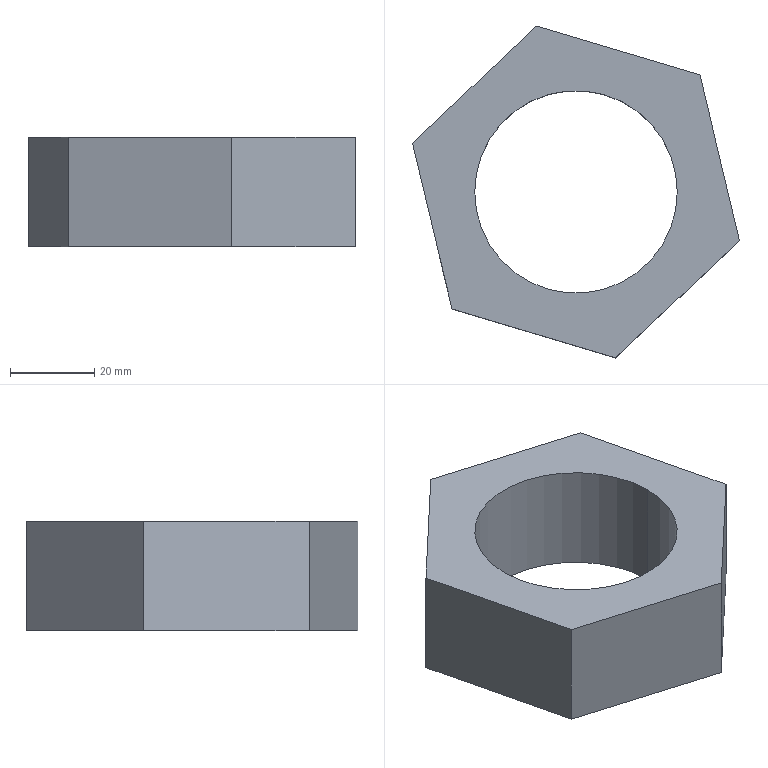Part | SolidWorks | features Extrusion 1 | 1 solid | 10 faces | box 77.461 x 78.628 x 26 mm | volume 63283 mm3 | plane 8 | cylinder 2 | commonest cylinder face diameters 48 x2
STEP:
#1=CARTESIAN_POINT('',(-24.,0.,26.));
#2=VERTEX_POINT('',#1);
#3=CARTESIAN_POINT('',(24.,0.,26.));
#4=VERTEX_POINT('',#3);
#5=CARTESIAN_POINT('',(0.,0.,26.));
#6=DIRECTION('',(0.,0.,1.));
#7=DIRECTION('',(1.,0.,0.));
#8=AXIS2_PLACEMENT_3D('',#5,#6,#7);
#9=CIRCLE('',#8,24.);
#10=EDGE_CURVE('',#2,#4,#9,.T.);
#11=ORIENTED_EDGE('',*,*,#10,.T.);
#12=CARTESIAN_POINT('',(24.,0.,0.));
#13=VERTEX_POINT('',#12);
#14=CARTESIAN_POINT('',(24.,0.,26.));
#15=DIRECTION('',(0.,0.,-1.));
#16=VECTOR('',#15,1000.);
#17=LINE('',#14,#16);
#18=EDGE_CURVE('',#4,#13,#17,.T.);
#19=ORIENTED_EDGE('',*,*,#18,.T.);
#20=CARTESIAN_POINT('',(-24.,0.,0.));
#21=VERTEX_POINT('',#20);
#22=CARTESIAN_POINT('',(0.,0.,0.));
#23=DIRECTION('',(0.,0.,1.));
#24=DIRECTION('',(1.,0.,0.));
#25=AXIS2_PLACEMENT_3D('',#22,#23,#24);
#26=CIRCLE('',#25,24.);
#27=EDGE_CURVE('',#21,#13,#26,.T.);
#28=ORIENTED_EDGE('',*,*,#27,.F.);
#29=CARTESIAN_POINT('',(-24.,0.,26.));
#30=DIRECTION('',(0.,0.,-1.));
#31=VECTOR('',#30,1000.);
#32=LINE('',#29,#31);
#33=EDGE_CURVE('',#2,#21,#32,.T.);
#34=ORIENTED_EDGE('',*,*,#33,.F.);
#35=EDGE_LOOP('',(#11,#19,#28,#34));
#36=FACE_OUTER_BOUND('',#35,.T.);
#37=CARTESIAN_POINT('',(0.,0.,26.));
#38=DIRECTION('',(0.,0.,-1.));
#39=DIRECTION('',(-1.,0.,0.));
#40=AXIS2_PLACEMENT_3D('',#37,#38,#39);
#41=CYLINDRICAL_SURFACE('',#40,24.);
#42=ADVANCED_FACE('',(#36),#41,.F.);
#43=CARTESIAN_POINT('',(9.367,-39.314,26.));
#44=VERTEX_POINT('',#43);
#45=CARTESIAN_POINT('',(38.731,-11.545,26.));
#46=VERTEX_POINT('',#45);
#47=CARTESIAN_POINT('',(9.367,-39.314,26.));
#48=DIRECTION('',(0.7266,0.6871,0.));
#49=VECTOR('',#48,1000.);
#50=LINE('',#47,#49);
#51=EDGE_CURVE('',#44,#46,#50,.T.);
#52=ORIENTED_EDGE('',*,*,#51,.T.);
#53=CARTESIAN_POINT('',(29.363,27.769,26.));
#54=VERTEX_POINT('',#53);
#55=CARTESIAN_POINT('',(38.731,-11.545,26.));
#56=DIRECTION('',(-0.2318,0.9728,0.));
#57=VECTOR('',#56,1000.);
#58=LINE('',#55,#57);
#59=EDGE_CURVE('',#46,#54,#58,.T.);
#60=ORIENTED_EDGE('',*,*,#59,.T.);
#61=CARTESIAN_POINT('',(-9.367,39.314,26.));
#62=VERTEX_POINT('',#61);
#63=CARTESIAN_POINT('',(29.363,27.769,26.));
#64=DIRECTION('',(-0.9583,0.2857,0.));
#65=VECTOR('',#64,1000.);
#66=LINE('',#63,#65);
#67=EDGE_CURVE('',#54,#62,#66,.T.);
#68=ORIENTED_EDGE('',*,*,#67,.T.);
#69=CARTESIAN_POINT('',(-38.731,11.545,26.));
#70=VERTEX_POINT('',#69);
#71=CARTESIAN_POINT('',(-9.367,39.314,26.));
#72=DIRECTION('',(-0.7266,-0.6871,0.));
#73=VECTOR('',#72,1000.);
#74=LINE('',#71,#73);
#75=EDGE_CURVE('',#62,#70,#74,.T.);
#76=ORIENTED_EDGE('',*,*,#75,.T.);
#77=CARTESIAN_POINT('',(-29.363,-27.769,26.));
#78=VERTEX_POINT('',#77);
#79=CARTESIAN_POINT('',(-38.731,11.545,26.));
#80=DIRECTION('',(0.2318,-0.9728,0.));
#81=VECTOR('',#80,1000.);
#82=LINE('',#79,#81);
#83=EDGE_CURVE('',#70,#78,#82,.T.);
#84=ORIENTED_EDGE('',*,*,#83,.T.);
#85=CARTESIAN_POINT('',(-29.363,-27.769,26.));
#86=DIRECTION('',(0.9583,-0.2857,0.));
#87=VECTOR('',#86,1000.);
#88=LINE('',#85,#87);
#89=EDGE_CURVE('',#78,#44,#88,.T.);
#90=ORIENTED_EDGE('',*,*,#89,.T.);
#91=EDGE_LOOP('',(#52,#60,#68,#76,#84,#90));
#92=FACE_OUTER_BOUND('',#91,.T.);
#93=ORIENTED_EDGE('',*,*,#10,.F.);
#94=CARTESIAN_POINT('',(0.,0.,26.));
#95=DIRECTION('',(0.,0.,1.));
#96=DIRECTION('',(1.,0.,0.));
#97=AXIS2_PLACEMENT_3D('',#94,#95,#96);
#98=CIRCLE('',#97,24.);
#99=EDGE_CURVE('',#4,#2,#98,.T.);
#100=ORIENTED_EDGE('',*,*,#99,.F.);
#101=EDGE_LOOP('',(#93,#100));
#102=FACE_BOUND('',#101,.T.);
#103=CARTESIAN_POINT('',(0.,0.,26.));
#104=DIRECTION('',(0.,0.,1.));
#105=DIRECTION('',(1.,0.,0.));
#106=AXIS2_PLACEMENT_3D('',#103,#104,#105);
#107=PLANE('',#106);
#108=ADVANCED_FACE('',(#92,#102),#107,.T.);
#109=CARTESIAN_POINT('',(9.367,-39.314,0.));
#110=VERTEX_POINT('',#109);
#111=CARTESIAN_POINT('',(38.731,-11.545,0.));
#112=VERTEX_POINT('',#111);
#113=CARTESIAN_POINT('',(9.367,-39.314,0.));
#114=DIRECTION('',(0.7266,0.6871,0.));
#115=VECTOR('',#114,1000.);
#116=LINE('',#113,#115);
#117=EDGE_CURVE('',#110,#112,#116,.T.);
#118=ORIENTED_EDGE('',*,*,#117,.F.);
#119=CARTESIAN_POINT('',(-29.363,-27.769,0.));
#120=VERTEX_POINT('',#119);
#121=CARTESIAN_POINT('',(-29.363,-27.769,0.));
#122=DIRECTION('',(0.9583,-0.2857,0.));
#123=VECTOR('',#122,1000.);
#124=LINE('',#121,#123);
#125=EDGE_CURVE('',#120,#110,#124,.T.);
#126=ORIENTED_EDGE('',*,*,#125,.F.);
#127=CARTESIAN_POINT('',(-38.731,11.545,0.));
#128=VERTEX_POINT('',#127);
#129=CARTESIAN_POINT('',(-38.731,11.545,0.));
#130=DIRECTION('',(0.2318,-0.9728,0.));
#131=VECTOR('',#130,1000.);
#132=LINE('',#129,#131);
#133=EDGE_CURVE('',#128,#120,#132,.T.);
#134=ORIENTED_EDGE('',*,*,#133,.F.);
#135=CARTESIAN_POINT('',(-9.367,39.314,0.));
#136=VERTEX_POINT('',#135);
#137=CARTESIAN_POINT('',(-9.367,39.314,0.));
#138=DIRECTION('',(-0.7266,-0.6871,0.));
#139=VECTOR('',#138,1000.);
#140=LINE('',#137,#139);
#141=EDGE_CURVE('',#136,#128,#140,.T.);
#142=ORIENTED_EDGE('',*,*,#141,.F.);
#143=CARTESIAN_POINT('',(29.363,27.769,0.));
#144=VERTEX_POINT('',#143);
#145=CARTESIAN_POINT('',(29.363,27.769,0.));
#146=DIRECTION('',(-0.9583,0.2857,0.));
#147=VECTOR('',#146,1000.);
#148=LINE('',#145,#147);
#149=EDGE_CURVE('',#144,#136,#148,.T.);
#150=ORIENTED_EDGE('',*,*,#149,.F.);
#151=CARTESIAN_POINT('',(38.731,-11.545,0.));
#152=DIRECTION('',(-0.2318,0.9728,0.));
#153=VECTOR('',#152,1000.);
#154=LINE('',#151,#153);
#155=EDGE_CURVE('',#112,#144,#154,.T.);
#156=ORIENTED_EDGE('',*,*,#155,.F.);
#157=EDGE_LOOP('',(#118,#126,#134,#142,#150,#156));
#158=FACE_OUTER_BOUND('',#157,.T.);
#159=ORIENTED_EDGE('',*,*,#27,.T.);
#160=CARTESIAN_POINT('',(0.,0.,0.));
#161=DIRECTION('',(0.,0.,1.));
#162=DIRECTION('',(1.,0.,0.));
#163=AXIS2_PLACEMENT_3D('',#160,#161,#162);
#164=CIRCLE('',#163,24.);
#165=EDGE_CURVE('',#13,#21,#164,.T.);
#166=ORIENTED_EDGE('',*,*,#165,.T.);
#167=EDGE_LOOP('',(#159,#166));
#168=FACE_BOUND('',#167,.T.);
#169=CARTESIAN_POINT('',(0.,0.,0.));
#170=DIRECTION('',(0.,0.,1.));
#171=DIRECTION('',(1.,0.,0.));
#172=AXIS2_PLACEMENT_3D('',#169,#170,#171);
#173=PLANE('',#172);
#174=ADVANCED_FACE('',(#158,#168),#173,.F.);
#175=ORIENTED_EDGE('',*,*,#117,.T.);
#176=CARTESIAN_POINT('',(38.731,-11.545,26.));
#177=DIRECTION('',(0.,0.,-1.));
#178=VECTOR('',#177,1000.);
#179=LINE('',#176,#178);
#180=EDGE_CURVE('',#46,#112,#179,.T.);
#181=ORIENTED_EDGE('',*,*,#180,.F.);
#182=ORIENTED_EDGE('',*,*,#51,.F.);
#183=CARTESIAN_POINT('',(9.367,-39.314,26.));
#184=DIRECTION('',(0.,0.,-1.));
#185=VECTOR('',#184,1000.);
#186=LINE('',#183,#185);
#187=EDGE_CURVE('',#44,#110,#186,.T.);
#188=ORIENTED_EDGE('',*,*,#187,.T.);
#189=EDGE_LOOP('',(#175,#181,#182,#188));
#190=FACE_OUTER_BOUND('',#189,.T.);
#191=CARTESIAN_POINT('',(9.367,-39.314,26.));
#192=DIRECTION('',(-0.6871,0.7266,0.));
#193=DIRECTION('',(-0.7266,-0.6871,0.));
#194=AXIS2_PLACEMENT_3D('',#191,#192,#193);
#195=PLANE('',#194);
#196=ADVANCED_FACE('',(#190),#195,.F.);
#197=ORIENTED_EDGE('',*,*,#155,.T.);
#198=CARTESIAN_POINT('',(29.363,27.769,26.));
#199=DIRECTION('',(0.,0.,-1.));
#200=VECTOR('',#199,1000.);
#201=LINE('',#198,#200);
#202=EDGE_CURVE('',#54,#144,#201,.T.);
#203=ORIENTED_EDGE('',*,*,#202,.F.);
#204=ORIENTED_EDGE('',*,*,#59,.F.);
#205=ORIENTED_EDGE('',*,*,#180,.T.);
#206=EDGE_LOOP('',(#197,#203,#204,#205));
#207=FACE_OUTER_BOUND('',#206,.T.);
#208=CARTESIAN_POINT('',(38.731,-11.545,26.));
#209=DIRECTION('',(-0.9728,-0.2318,0.));
#210=DIRECTION('',(0.2318,-0.9728,0.));
#211=AXIS2_PLACEMENT_3D('',#208,#209,#210);
#212=PLANE('',#211);
#213=ADVANCED_FACE('',(#207),#212,.F.);
#214=ORIENTED_EDGE('',*,*,#149,.T.);
#215=CARTESIAN_POINT('',(-9.367,39.314,26.));
#216=DIRECTION('',(0.,0.,-1.));
#217=VECTOR('',#216,1000.);
#218=LINE('',#215,#217);
#219=EDGE_CURVE('',#62,#136,#218,.T.);
#220=ORIENTED_EDGE('',*,*,#219,.F.);
#221=ORIENTED_EDGE('',*,*,#67,.F.);
#222=ORIENTED_EDGE('',*,*,#202,.T.);
#223=EDGE_LOOP('',(#214,#220,#221,#222));
#224=FACE_OUTER_BOUND('',#223,.T.);
#225=CARTESIAN_POINT('',(29.363,27.769,26.));
#226=DIRECTION('',(-0.2857,-0.9583,0.));
#227=DIRECTION('',(0.9583,-0.2857,0.));
#228=AXIS2_PLACEMENT_3D('',#225,#226,#227);
#229=PLANE('',#228);
#230=ADVANCED_FACE('',(#224),#229,.F.);
#231=ORIENTED_EDGE('',*,*,#141,.T.);
#232=CARTESIAN_POINT('',(-38.731,11.545,26.));
#233=DIRECTION('',(0.,0.,-1.));
#234=VECTOR('',#233,1000.);
#235=LINE('',#232,#234);
#236=EDGE_CURVE('',#70,#128,#235,.T.);
#237=ORIENTED_EDGE('',*,*,#236,.F.);
#238=ORIENTED_EDGE('',*,*,#75,.F.);
#239=ORIENTED_EDGE('',*,*,#219,.T.);
#240=EDGE_LOOP('',(#231,#237,#238,#239));
#241=FACE_OUTER_BOUND('',#240,.T.);
#242=CARTESIAN_POINT('',(-9.367,39.314,26.));
#243=DIRECTION('',(0.6871,-0.7266,0.));
#244=DIRECTION('',(0.7266,0.6871,0.));
#245=AXIS2_PLACEMENT_3D('',#242,#243,#244);
#246=PLANE('',#245);
#247=ADVANCED_FACE('',(#241),#246,.F.);
#248=ORIENTED_EDGE('',*,*,#133,.T.);
#249=CARTESIAN_POINT('',(-29.363,-27.769,26.));
#250=DIRECTION('',(0.,0.,-1.));
#251=VECTOR('',#250,1000.);
#252=LINE('',#249,#251);
#253=EDGE_CURVE('',#78,#120,#252,.T.);
#254=ORIENTED_EDGE('',*,*,#253,.F.);
#255=ORIENTED_EDGE('',*,*,#83,.F.);
#256=ORIENTED_EDGE('',*,*,#236,.T.);
#257=EDGE_LOOP('',(#248,#254,#255,#256));
#258=FACE_OUTER_BOUND('',#257,.T.);
#259=CARTESIAN_POINT('',(-38.731,11.545,26.));
#260=DIRECTION('',(0.9728,0.2318,0.));
#261=DIRECTION('',(-0.2318,0.9728,0.));
#262=AXIS2_PLACEMENT_3D('',#259,#260,#261);
#263=PLANE('',#262);
#264=ADVANCED_FACE('',(#258),#263,.F.);
#265=ORIENTED_EDGE('',*,*,#125,.T.);
#266=ORIENTED_EDGE('',*,*,#187,.F.);
#267=ORIENTED_EDGE('',*,*,#89,.F.);
#268=ORIENTED_EDGE('',*,*,#253,.T.);
#269=EDGE_LOOP('',(#265,#266,#267,#268));
#270=FACE_OUTER_BOUND('',#269,.T.);
#271=CARTESIAN_POINT('',(-29.363,-27.769,26.));
#272=DIRECTION('',(0.2857,0.9583,0.));
#273=DIRECTION('',(-0.9583,0.2857,0.));
#274=AXIS2_PLACEMENT_3D('',#271,#272,#273);
#275=PLANE('',#274);
#276=ADVANCED_FACE('',(#270),#275,.F.);
#277=ORIENTED_EDGE('',*,*,#18,.F.);
#278=ORIENTED_EDGE('',*,*,#99,.T.);
#279=ORIENTED_EDGE('',*,*,#33,.T.);
#280=ORIENTED_EDGE('',*,*,#165,.F.);
#281=EDGE_LOOP('',(#277,#278,#279,#280));
#282=FACE_OUTER_BOUND('',#281,.T.);
#283=CARTESIAN_POINT('',(0.,0.,26.));
#284=DIRECTION('',(0.,0.,-1.));
#285=DIRECTION('',(-1.,0.,0.));
#286=AXIS2_PLACEMENT_3D('',#283,#284,#285);
#287=CYLINDRICAL_SURFACE('',#286,24.);
#288=ADVANCED_FACE('',(#282),#287,.F.);
#289=CLOSED_SHELL('',(#42,#108,#174,#196,#213,#230,#247,#264,#276,#288));
#290=MANIFOLD_SOLID_BREP('',#289);
#291=CARTESIAN_POINT('',(0.,0.,0.));
#292=DIRECTION('',(0.,0.,1.));
#293=DIRECTION('',(1.,0.,0.));
#294=AXIS2_PLACEMENT_3D('',#291,#292,#293);
#295=(LENGTH_UNIT()NAMED_UNIT(*)SI_UNIT(.MILLI.,.METRE.));
#296=UNCERTAINTY_MEASURE_WITH_UNIT(LENGTH_MEASURE(0.00001),#295,'','');
#297=(NAMED_UNIT(*)PLANE_ANGLE_UNIT()SI_UNIT($,.RADIAN.));
#298=(NAMED_UNIT(*)SI_UNIT($,.STERADIAN.)SOLID_ANGLE_UNIT());
#299=(GEOMETRIC_REPRESENTATION_CONTEXT(3)GLOBAL_UNCERTAINTY_ASSIGNED_CONTEXT((#296))GLOBAL_UNIT_ASSIGNED_CONTEXT((#295,#297,#298))REPRESENTATION_CONTEXT('',''));
#300=ADVANCED_BREP_SHAPE_REPRESENTATION('',(#290,#294),#299);